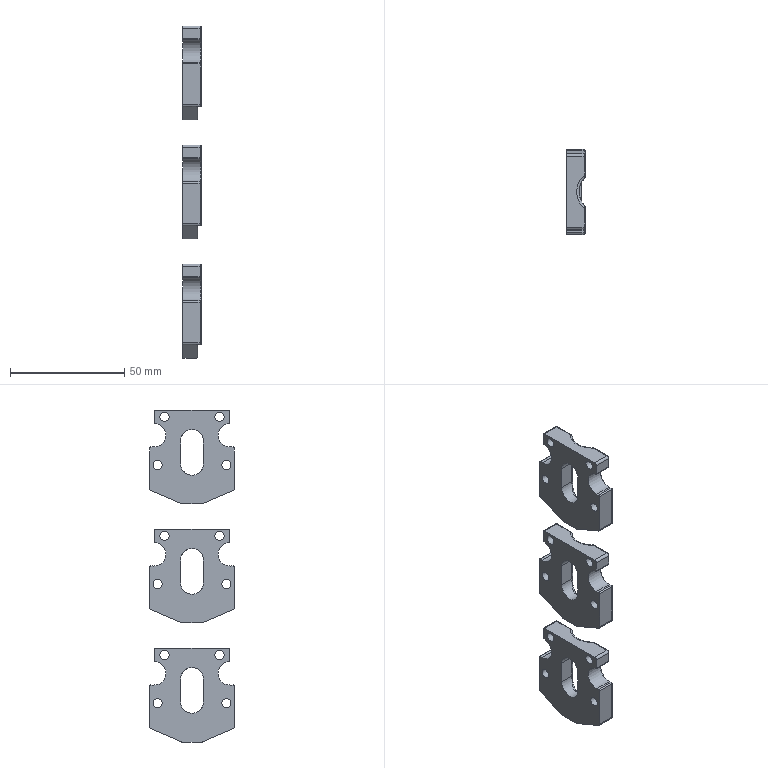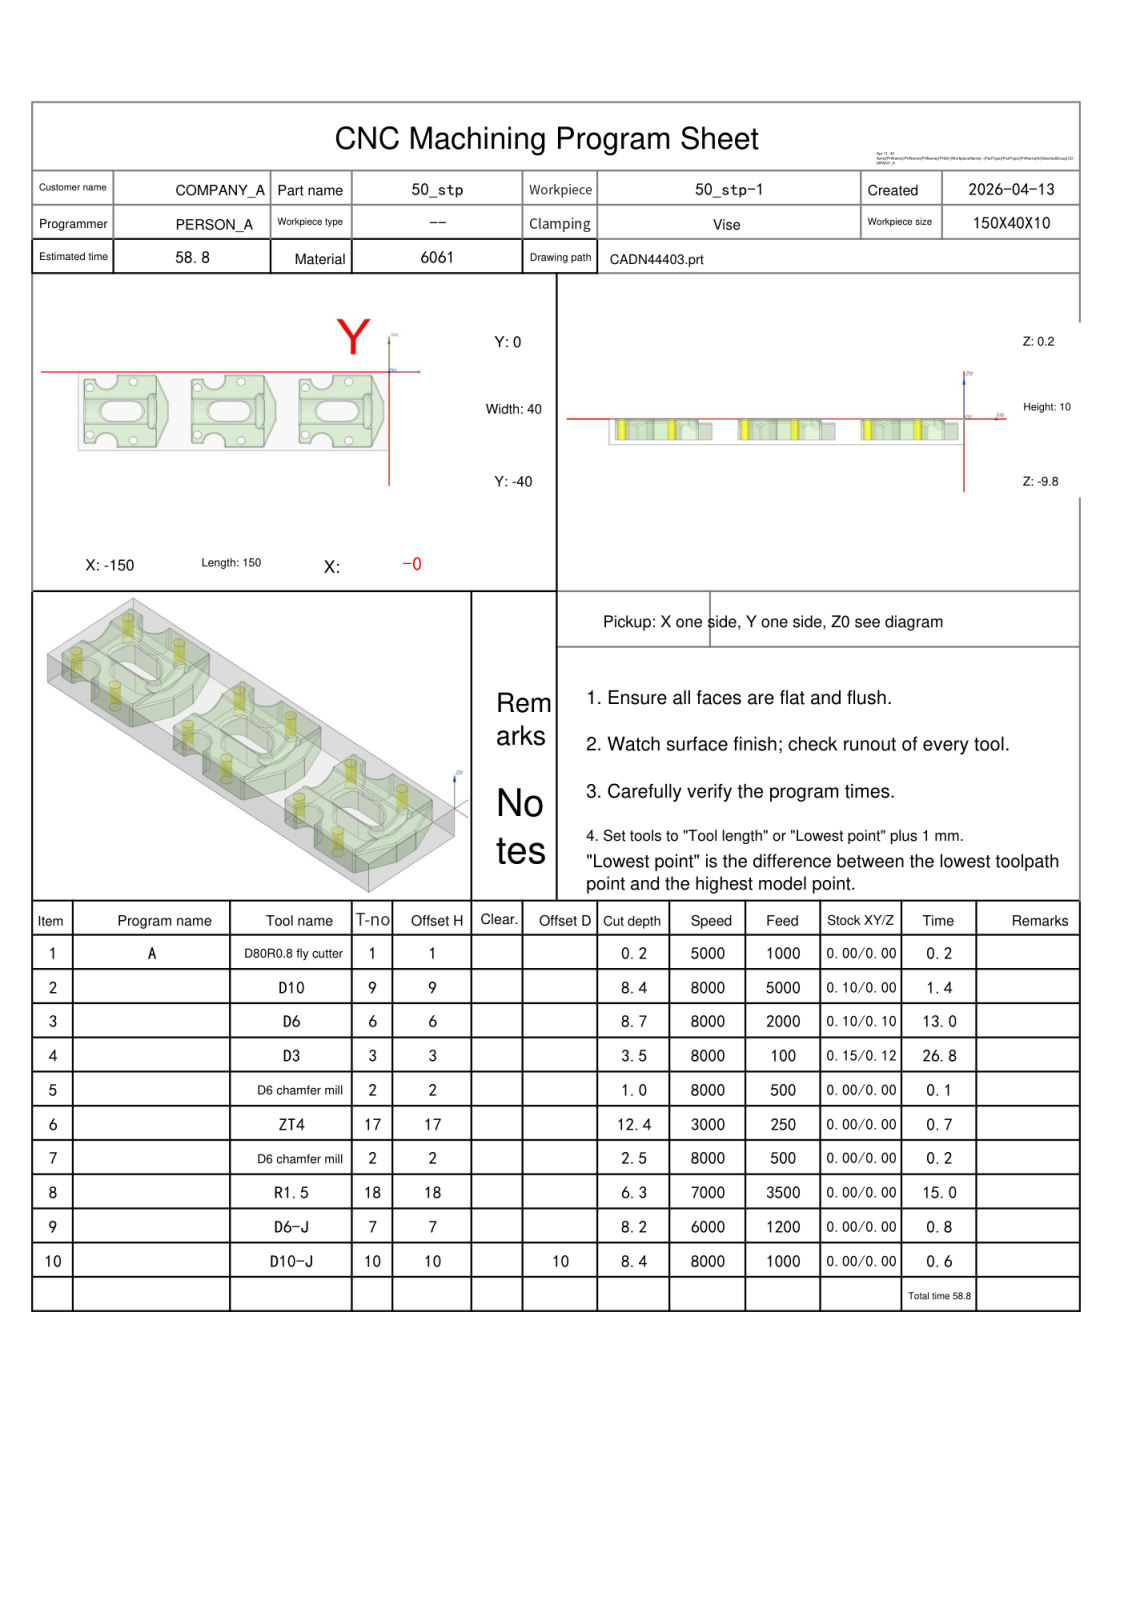NC program | NX | posted by the shop | part box 8 x 37 x 145 mm
Lines 15399 to 16378 of 223411:
N4 T03 M06
(D3  D=3. R=0. H=03 ce=0.15 di=0.12)
G00 G90 G54 X-112.073 Y-14.319 M03 S8000
G43 H03 Z10.15
M08
Z.405
G01 Z-.095 F100.
G03 X-113.572 Y-12.853 I-1.5 J-.034
G01 X-114.3
G03 X-114.703 Y-13.422 I.341 J-.668
G02 X-114.826 Y-13.87 I-3.495 J.718
G03 X-114.908 Y-14.36 I1.418 J-.49
X-114.117 Y-15.682 I1.5 J0.0
G01 Z.405
G00 Z3.
G01 X-111.94 Y-14.368 F6000.
G00 Z.31
G01 Z-.19 F100.
G03 X-113.439 Y-12.924 I-1.499 J-.057
G01 X-114.306
G03 X-114.705 Y-13.731 I.775 J-.885
G01 X-114.72 Y-13.816
G03 X-114.748 Y-14.107 I1.471 J-.291
X-113.834 Y-15.488 I1.5 J0.0
G01 Z.31
G00 Z2.905
G01 X-111.919 Y-14.435 F6000.
G00 Z.215
G01 Z-.285 F100.
G03 X-113.418 Y-12.994 I-1.499 J-.059
G01 X-114.298
G03 X-114.581 Y-13.422 I.509 J-.643
G01 X-114.698 Y-13.877
G03 X-114.745 Y-14.251 I1.453 J-.374
X-113.843 Y-15.626 I1.5 J0.0
G01 Z.215
G00 Z2.81
G01 X-112.162 Y-14.542 F6000.
G00 Z.12
G01 Z-.38 F100.
G03 X-113.662 Y-13.065 I-1.5 J-.023
G01 X-114.3
G03 X-114.663 Y-13.852 I.965 J-.922
G01 X-114.671 Y-14.004
G03 X-113.644 Y-15.428 I1.5 J0.0
G01 Z.12
G00 Z2.715
G01 X-111.678 Y-14.54 F6000.
G00 Z.025
G01 Z-.475 F100.
G03 X-113.175 Y-13.138 I-1.497 J-.098
G01 X-114.3
G03 X-114.635 Y-13.846 I.905 J-.861
G02 X-114.675 Y-14.063 I-2.625 J.378
G03 X-114.713 Y-14.399 I1.462 J-.336
X-113.808 Y-15.776 I1.5 J0.0
G01 Z.025
G00 Z2.62
G01 X-112.076 Y-14.687 F6000.
G00 Z-.07
G01 Z-.57 F100.
G03 X-113.576 Y-13.213 I-1.5 J-.026
G01 X-114.3
G03 X-114.607 Y-13.846 I.884 J-.82
G01 X-114.645 Y-14.013
G03 X-114.681 Y-14.34 I1.464 J-.327
X-113.696 Y-15.749 I1.5 J0.0
G01 Z-.07
G00 Z2.525
G01 X-112.279 Y-14.78 F6000.
G00 Z-.165
G01 Z-.665 F100.
G03 X-113.779 Y-13.29 I-1.5 J-.01
G01 X-114.254
G03 X-114.578 Y-13.846 I.496 J-.661
G01 X-114.594 Y-13.952
G03 X-114.616 Y-14.207 I1.478 J-.255
X-113.595 Y-15.629 I1.5 J0.0
G01 Z-.165
G00 Z2.43
G01 X-111.613 Y-14.745 F6000.
G00 Z-.26
G01 Z-.76 F100.
G03 X-113.107 Y-13.376 I-1.494 J-.131
G01 X-114.274
G03 X-114.593 Y-13.946 I1.157 J-1.022
G01 X-114.65 Y-14.212
X-114.656 Y-14.271
G02 X-114.763 Y-14.734 I-2.214 J.269
G03 X-114.846 Y-15.227 I1.417 J-.493
X-114.108 Y-16.519 I1.5 J0.0
G01 Z-.26
G00 Z2.335
G01 X-111.422 Y-14.809 F6000.
G00 Z-.355
G01 Z-.855 F100.
G03 X-112.913 Y-13.476 I-1.491 J-.166
G01 X-113.979
X-114.287 Y-13.472
G03 X-114.632 Y-14.271 I1.061 J-.933
G02 X-114.704 Y-14.623 I-2.621 J.349
G03 X-114.757 Y-15.02 I1.446 J-.397
X-113.91 Y-16.371 I1.5 J0.0
G01 Z-.355
G00 Z2.24
G01 X-109.207 Y-12.251 F6000.
G00 Z-.45
G01 Z-.95 F100.
G03 X-109.78 Y-12.137 I-.573 J-1.386
X-111.015 Y-12.786 I0.0 J-1.5
G02 X-112.167 Y-13.603 I-1.698 J1.171
G01 X-112.5 Y-13.591
X-113.644
X-114.289 Y-13.563
G03 X-114.609 Y-14.271 I.917 J-.841
G02 X-114.679 Y-14.618 I-3.409 J.509
G03 X-114.726 Y-14.991 I1.453 J-.373
X-113.815 Y-16.37 I1.5 J0.0
G01 Z-.45
G00 Z2.145
G01 X-111.691 Y-15.135 F6000.
G00 Z-.545
G01 Z-1.045 F100.
X-111.71 Y-15.004
G03 X-113.195 Y-13.718 I-1.485 J-.214
X-113.409 Y-13.733 I0.0 J-1.5
G01 X-113.436 Y-13.737
X-114.291 Y-13.652
G03 X-114.581 Y-14.271 I.881 J-.791
G02 X-114.639 Y-14.576 I-3.937 J.582
G03 X-114.676 Y-14.91 I1.462 J-.334
X-113.708 Y-16.313 I1.5 J0.0
G01 Z-.545
G00 Z2.05
G01 X-109.15 Y-11.698 F6000.
G00 Z-.64
G01 Z-1.14 F100.
G03 X-109.407 Y-11.676 I-.257 J-1.478
X-110.808 Y-12.64 I0.0 J-1.5
G02 X-111.321 Y-13.447 I-2.242 J.858
X-112.423 Y-13.903 I-1.102 J1.105
G01 X-112.5 Y-13.901
X-113.346
X-113.436 Y-13.921
X-114.292 Y-13.742
G03 X-114.65 Y-14.695 I1.567 J-1.133
G02 X-114.75 Y-15.15 I-2.534 J.317
G03 X-114.82 Y-15.603 I1.43 J-.453
X-114.008 Y-16.936 I1.5 J0.0
G01 Z-.64
G00 Z1.955
G01 X-109.437 Y-13.422 F6000.
G00 Z-.735
G01 Z-1.235 F100.
G03 X-110.228 Y-13.196 I-.79 J-1.275
X-111.286 Y-13.634 I0.0 J-1.5
G02 X-112.499 Y-14.135 I-1.213 J1.218
G01 X-113.353
G02 X-114.292 Y-13.832 I0.0 J1.608
G03 X-114.626 Y-14.695 I1.455 J-1.058
G02 X-114.712 Y-15.11 I-3.389 J.489
G03 X-114.765 Y-15.506 I1.447 J-.396
X-113.882 Y-16.873 I1.5 J0.0
G01 Z-.735
G00 Z1.86
G01 X-112.717 Y-16.057 F6000.
G00 Z-.83
G01 Z-1.33 F100.
G03 X-112.675 Y-15.704 I-1.458 J.353
X-113.443 Y-14.395 I-1.5 J0.0
G01 X-114.291 Y-13.921
G03 X-114.603 Y-14.695 I1.227 J-.946
G02 X-114.672 Y-15.073 I-3.674 J.471
G03 X-114.712 Y-15.417 I1.46 J-.344
X-113.762 Y-16.813 I1.5 J0.0
G01 Z-.83
G00 Z1.765
G01 X-115.362 Y-19.956 F6000.
G00 Z-.929
G01 Z-1.429 F100.
G03 X-113.862 Y-18.456 I0.0 J1.5
G01 Y-15.844
X-113.86 Y-15.711
G03 X-114.022 Y-14.531 I-4.374 J0.0
X-114.297 Y-14.039 I-1.16 J-.325
X-114.657 Y-15.12 I1.993 J-1.265
G02 X-115.551 Y-16.809 I-2.718 J.357
X-116.686 Y-17.228 I-1.135 J1.331
G01 X-116.794 Y-17.224
G03 X-118.294 Y-18.724 I0.0 J-1.5
G01 Y-18.847
Z-.929
G00 Z1.67
G01 X-115.426 Y-19.782 F6000.
G00 Z-1.028
G01 Z-1.528 F100.
G03 X-113.926 Y-18.282 I0.0 J1.5
G01 Y-15.844
Y-15.836
G03 X-114.041 Y-14.695 I-5.707 J0.0
X-114.296 Y-14.147 I-1.32 J-.28
X-114.631 Y-15.12 I2.026 J-1.24
G02 X-115.479 Y-16.914 I-2.978 J.31
X-115.953 Y-17.248 I-1.174 J1.16
G03 X-116.817 Y-18.607 I.636 J-1.358
X-116.788 Y-18.901 I1.5 J0.0
G01 Z-1.028
G00 Z1.571
G01 X-115.449 Y-20.075 F6000.
G00 Z-1.127
G01 Z-1.627 F100.
G03 X-113.949 Y-18.575 I0.0 J1.5
G01 Y-15.657
G03 X-114.282 Y-14.274 I-3.038 J0.0
G01 X-114.308 Y-14.271
X-114.507 Y-14.695
X-114.68 Y-15.544
G02 X-115.469 Y-17.081 I-2.826 J.481
X-116.693 Y-17.592 I-1.223 J1.209
G01 X-116.794 Y-17.589
G03 X-118.295 Y-19.089 I0.0 J-1.501
G01 X-118.294 Y-19.142
Z-1.127
G00 Z1.472
G01 X-115.45 Y-20.345 F6000.
G00 Z-1.226
G01 Z-1.726 F100.
G03 X-113.95 Y-18.845 I0.0 J1.5
G01 X-113.949 Y-15.994
Y-15.807
G03 X-114.282 Y-14.401 I-3.533 J-.093
X-114.573 Y-15.12 I.91 J-.787
G02 X-115.099 Y-16.817 I-4.444 J.448
X-116.777 Y-17.788 I-1.678 J.965
G01 X-116.794
G03 X-118.294 Y-19.288 I0.0 J-1.5
G01 Y-19.291
Z-1.226
G00 Z1.373
G01 X-115.45 Y-20.496 F6000.
G00 Z-1.326
G01 Z-1.826 F100.
G03 X-113.95 Y-18.996 I0.0 J1.5
G01 Y-16.074
X-114.059 Y-15.12
X-114.282 Y-14.527
X-114.311 Y-14.522
G03 X-114.624 Y-15.544 I2.7 J-1.384
G02 X-115.449 Y-17.465 I-3.252 J.258
X-116.302 Y-17.965 I-1.207 J1.084
G03 X-117.474 Y-19.429 I.327 J-1.464
G01 X-117.472 Y-19.501
Z-1.326
G00 Z2.525
G01 X-111.599 Y-14.741 F6000.
G00 Z-.26
G01 Z-.76 F100.
X-112.853 Y-14.174
G03 X-113.471 Y-14.04 I-.619 J-1.366
X-114.838 Y-14.922 I0.0 J-1.5
G02 X-116.796 Y-16.229 I-2.031 J.922
G03 X-118.296 Y-17.729 I0.0 J-1.5
G01 Y-17.74
Z-.26
G00 Z3.
G01 X-114.081 Y-24.359 F6000.
G00 Z.405
G01 Z-.095 F100.
G03 X-114.902 Y-25.697 I.678 J-1.338
X-114.826 Y-26.171 I1.5 J0.0
G01 X-114.584 Y-26.896
X-114.349 Y-27.131
X-114.3 Y-27.147
X-113.57
G03 X-112.071 Y-25.681 I0.0 J1.5
G01 Z.405
G00 Z3.
G01 X-113.871 Y-24.459 F6000.
G00 Z.31
G01 Z-.19 F100.
G03 X-114.762 Y-25.83 I.609 J-1.371
X-114.728 Y-26.147 I1.5 J0.0
G01 X-114.695 Y-26.341
G03 X-114.3 Y-27.076 I1.143 J.141
G01 X-113.461
G03 X-111.962 Y-25.628 I0.0 J1.5
G01 Z.31
G00 Z2.905
G01 X-118.286 Y-22.261 F6000.
G00 Z-.26
G01 Z-.76 F100.
Y-22.271
G03 X-116.786 Y-23.771 I1.5 J0.0
G01 X-116.749
G02 X-114.842 Y-25.07 I-.121 J-2.228
G03 X-113.478 Y-25.946 I1.364 J.624
X-112.854 Y-25.81 I0.0 J1.5
G01 X-111.629 Y-25.25
Z-.26
G00 Z2.81
G01 X-113.777 Y-24.47 F6000.
G00 Z.215
G01 Z-.285 F100.
G03 X-114.718 Y-25.862 I.559 J-1.392
X-114.695 Y-26.126 I1.5 J0.0
G01 X-114.678 Y-26.236
G03 X-114.299 Y-27.006 I1.304 J.164
G01 X-113.439
G03 X-111.94 Y-25.561 I0.0 J1.5
G01 Z.215
G00 Z2.81
G01 X-113.713 Y-24.458 F6000.
G00 Z.12
G01 Z-.38 F100.
G03 X-114.689 Y-25.864 I.525 J-1.405
X-114.671 Y-26.093 I1.5 J0.0
G01 X-114.662 Y-26.154
G03 X-114.3 Y-26.935 I1.301 J.129
G01 X-113.602
G03 X-112.102 Y-25.463 I0.0 J1.5
G01 Z.12
G00 Z2.715
G01 X-113.812 Y-24.206 F6000.
G00 Z.025
G01 Z-.475 F100.
G03 X-114.72 Y-25.584 I.592 J-1.378
X-114.679 Y-25.933 I1.5 J0.0
G02 X-114.635 Y-26.154 I-2.825 J-.675
G03 X-114.3 Y-26.862 I1.22 J.144
G01 X-113.113
G03 X-111.618 Y-25.489 I0.0 J1.5
G01 Z.025
G00 Z2.62
G01 X-113.685 Y-24.306 F6000.
G00 Z-.07
G01 Z-.57 F100.
G03 X-114.66 Y-25.711 I.525 J-1.405
X-114.634 Y-25.993 I1.5 J0.0
G01 X-114.607 Y-26.154
G03 X-114.3 Y-26.787 I1.185 J.183
G01 X-113.577
G03 X-112.077 Y-25.318 I0.0 J1.5
G01 Z-.07
G00 Z2.525
G01 X-113.6 Y-24.361 F6000.
G00 Z-.165
G01 Z-.665 F100.
G03 X-114.618 Y-25.781 I.482 J-1.42
X-114.596 Y-26.041 I1.5 J0.0
G01 X-114.578 Y-26.154
G03 X-114.254 Y-26.71 I.817 J.103
G01 X-113.771
G03 X-112.271 Y-25.22 I0.0 J1.5
G01 Z-.165
G00 Z2.43
G01 X-114.106 Y-23.483 F6000.
G00 Z-.26
G01 Z-.76 F100.
G03 X-114.846 Y-24.776 I.76 J-1.293
X-114.763 Y-25.268 I1.5 J0.0
G02 X-114.656 Y-25.729 I-2.108 J-.731
G01 X-114.649 Y-25.791
X-114.595 Y-26.047
G03 X-114.285 Y-26.615 I1.52 J.459
G01 X-113.859 Y-26.624
X-113.199
G03 X-111.703 Y-25.23 I0.0 J1.5
G01 Z-.26
G00 Z2.335
G01 X-113.909 Y-23.613 F6000.
G00 Z-.355
G01 Z-.855 F100.
G03 X-114.767 Y-24.968 I.642 J-1.356
X-114.71 Y-25.378 I1.5 J0.0
G02 X-114.633 Y-25.729 I-2.929 J-.831
G03 X-114.287 Y-26.528 I1.409 J.136
G01 X-113.859 Y-26.516
X-113.794 Y-26.524
X-113.209
G03 X-111.712 Y-25.133 I0.0 J1.5
G01 Z-.355
G00 Z2.24
G01 X-113.813 Y-23.634 F6000.
G00 Z-.45
G01 Z-.95 F100.
G03 X-114.726 Y-25.014 I.587 J-1.38
X-114.679 Y-25.386 I1.5 J0.0
G02 X-114.609 Y-25.729 I-3.365 J-.862
G03 X-114.289 Y-26.437 I1.238 J.133
G01 X-113.614 Y-26.387
X-113.588 Y-26.409
X-112.5
G02 X-110.883 Y-27.437 I-.006 J-1.795
G03 X-109.521 Y-28.309 I1.362 J.628
X-109.154 Y-28.264 I0.0 J1.5
G01 Z-.45
G00 Z2.145
G01 X-113.701 Y-23.701 F6000.
G00 Z-.545
G01 Z-1.045 F100.
G03 X-114.673 Y-25.105 I.527 J-1.404
X-114.636 Y-25.436 I1.5 J0.0
G02 X-114.581 Y-25.729 I-3.903 J-.883
G03 X-114.291 Y-26.348 I1.171 J.173
G01 X-113.436 Y-26.263
X-113.392 Y-26.269
G03 X-113.18 Y-26.284 I.212 J1.485
X-111.695 Y-24.996 I0.0 J1.5
G01 X-111.677 Y-24.872
Z-.545
G00 Z2.05
G01 X-114.073 Y-22.957 F6000.
G00 Z-.64
G01 Z-1.14 F100.
G03 X-114.877 Y-24.286 I.695 J-1.329
X-114.793 Y-24.781 I1.5 J0.0
G02 X-114.551 Y-25.729 I-5.379 J-1.882
G03 X-114.292 Y-26.258 I1.065 J.193
G01 X-113.436 Y-26.073
X-113.301 Y-26.099
X-112.499
G02 X-110.901 Y-27.143 I0.0 J-1.744
G01 X-110.834 Y-27.312
G03 X-109.426 Y-28.294 I1.408 J.518
X-109.15 Y-28.268 I0.0 J1.5
G01 Z-.64
G00 Z1.955
G01 X-113.912 Y-23.087 F6000.
G00 Z-.735
G01 Z-1.235 F100.
G03 X-114.778 Y-24.446 I.635 J-1.359
X-114.72 Y-24.856 I1.5 J0.0
G02 X-114.626 Y-25.305 I-3.135 J-.892
G01 X-114.605 Y-25.448
X-114.59 Y-25.515
G03 X-114.292 Y-26.168 I1.756 J.407
G02 X-113.375 Y-25.865 I.918 J-1.239
G01 X-112.355
G02 X-111.477 Y-26.172 I0.0 J-1.413
G03 X-110.544 Y-26.497 I.933 J1.175
X-109.619 Y-26.179 I0.0 J1.5
G01 Z-.735
G00 Z1.86
G01 X-113.784 Y-23.15 F6000.
G00 Z-.83
G01 Z-1.33 F100.
G03 X-114.722 Y-24.541 I.562 J-1.391
X-114.679 Y-24.897 I1.5 J0.0
G02 X-114.603 Y-25.305 I-3.598 J-.879
G03 X-114.291 Y-26.079 I1.54 J.172
G01 X-113.425 Y-25.6
G03 X-112.651 Y-24.288 I-.726 J1.313
X-112.691 Y-23.943 I-1.5 J0.0
G01 Z-.83
G00 Z1.765
G01 X-118.287 Y-21.146 F6000.
G00 Z-.929
G01 Z-1.429 F100.
Y-21.276
G03 X-116.787 Y-22.776 I1.5 J0.0
G01 X-116.749
X-116.735
G02 X-115.259 Y-23.487 I0.0 J-1.888
X-114.657 Y-24.88 I-2.266 J-1.806
G03 X-114.296 Y-25.962 I2.35 J.183
X-114.011 Y-25.443 I-.856 J.809
X-113.861 Y-24.243 I-4.718 J1.2
G01 X-113.862 Y-24.156
Y-21.55
G03 X-115.362 Y-20.05 I-1.5 J0.0
G01 Z-.929
G00 Z1.67
G01 X-116.962 Y-21.099 F6000.
G00 Z-1.028
G01 Z-1.528 F100.
G03 X-116.982 Y-21.343 I1.48 J-.244
X-116.038 Y-22.736 I1.5 J0.0
G02 X-115.059 Y-23.607 I-.713 J-1.788
X-114.631 Y-24.88 I-3.046 J-1.733
G03 X-114.31 Y-25.835 I2.457 J.293
X-114.065 Y-25.437 I-.463 J.559
X-113.926 Y-24.192 I-5.484 J1.245
G01 Y-24.156
Y-21.72
G03 X-115.426 Y-20.22 I-1.5 J0.0
G01 Z-1.028
G00 Z1.571
G01 X-118.288 Y-20.767 F6000.
G00 Z-1.127
G01 Z-1.627 F100.
Y-20.911
G03 X-116.788 Y-22.411 I1.5 J0.0
G01 X-116.749
X-116.725
G02 X-115.245 Y-23.183 I0.0 J-1.806
X-114.604 Y-24.88 I-2.663 J-1.974
G03 X-114.311 Y-25.725 I2.106 J.259
G01 X-114.285 Y-25.729
G03 X-113.949 Y-24.355 I-2.647 J1.375
G01 Y-21.417
G03 X-115.449 Y-19.917 I-1.5 J0.0
G01 Z-1.127
G00 Z1.472
G01 X-118.288 Y-20.709 F6000.
G00 Z-1.226
G01 Z-1.726 F100.
Y-20.712
G03 X-116.788 Y-22.212 I1.5 J0.0
G01 X-116.749
G02 X-115.099 Y-23.183 I-.028 J-1.936
X-114.573 Y-24.88 I-3.918 J-2.145
G03 X-114.282 Y-25.599 I1.201 J.068
X-113.949 Y-24.182 I-3.223 J1.504
G01 X-113.95 Y-23.979
Y-21.083
G03 X-115.45 Y-19.583 I-1.5 J0.0
G01 Z-1.226
G00 Z1.373
G01 X-117.532 Y-20.499 F6000.
G00 Z-1.326
G01 Z-1.826 F100.
X-117.534 Y-20.578
G03 X-116.359 Y-22.042 I1.5 J0.0
G02 X-115.328 Y-22.684 I-.396 J-1.784
X-114.624 Y-24.456 I-2.54 J-2.035
G03 X-114.311 Y-25.478 I3.012 J.362
G01 X-114.282 Y-25.473
X-114.059 Y-24.88
X-113.958 Y-24.032
X-113.95 Y-23.926
Y-20.741
G03 X-115.45 Y-19.241 I-1.5 J0.0
G01 Y-19.393
Z-1.326
G00 Z1.274
G01 X-119.548 Y-20. F6000.
G00 Z-1.425
G01 Z-1.925 F100.
X-118.783 Y-19.823
G02 X-117.421 Y-18.952 I1.361 J-.63
X-116.792 Y-19.091 I0.0 J-1.5
G01 X-114.482 Y-20.159
G02 X-114.046 Y-20.84 I-.315 J-.681
X-114.796 Y-21.59 I-.75 J0.0
X-115.111 Y-21.521 I0.0 J.75
G01 X-116.543 Y-20.859
X-116.656 Y-20.834
G03 X-116.902 Y-20.992 I0.0 J-.27
G01 X-117.062 Y-21.345
X-117.088 Y-21.469
G03 X-116.788 Y-21.769 I.3 J0.0
G01 X-116.749
G02 X-115.128 Y-22.707 I-.032 J-1.926
X-114.595 Y-24.456 I-3.782 J-2.109
G03 X-114.312 Y-25.355 I2.386 J.257
G01 X-114.282 Y-25.346
X-114.103 Y-24.88
G03 X-113.95 Y-23.767 I-7.84 J1.642
G01 Y-16.233
G03 X-114.103 Y-15.12 I-8.037 J-.535
G01 X-114.282 Y-14.654
X-114.312 Y-14.645
G03 X-114.595 Y-15.544 I2.103 J-1.156
G02 X-115.128 Y-17.293 I-4.315 J.36
X-116.782 Y-18.231 I-1.654 J.988
G01 X-116.793
G03 X-118.293 Y-19.731 I0.0 J-1.5
G01 X-119.548 Y-20.
Z-1.425
G00 Z1.174
Z-1.524
G01 X-119.549 Z-2.024
X-117.957 Y-20.995
G02 X-117.988 Y-20.691 I1.469 J.303
X-116.792 Y-19.222 I1.5 J0.0
G01 X-114.897 Y-18.831
X-114.745 Y-18.815
G02 X-113.995 Y-19.565 I0.0 J-.75
X-114.593 Y-20.3 I-.75 J0.0
G01 X-116.688 Y-20.733
X-116.796 Y-20.743
X-116.857 Y-20.833
X-117.018 Y-21.025
G03 X-117.089 Y-21.218 I.229 J-.193
X-116.789 Y-21.518 I.3 J0.0
G01 X-116.749
G02 X-115.35 Y-22.201 I-.009 J-1.793
X-114.635 Y-24.032 I-2.656 J-2.092
G03 X-114.312 Y-25.223 I3.647 J.35
G01 X-114.282 Y-25.212
X-114.155 Y-24.88
G03 X-113.95 Y-23.555 I-5.26 J1.492
G01 Y-16.445
G03 X-114.155 Y-15.12 I-5.449 J-.164
G01 X-114.282 Y-14.788
X-114.312 Y-14.777
G03 X-114.635 Y-15.968 I3.324 J-1.541
G02 X-115.35 Y-17.799 I-3.371 J.262
X-116.758 Y-18.482 I-1.409 J1.109
G01 X-116.793
G03 X-118.293 Y-19.982 I0.0 J-1.5
G01 X-119.549 Y-20.
Z-1.524
G00 Z1.075
G01 X-120.764 Y-20.002 F6000.
G00 Z-1.623
G01 Z-2.123 F100.
X-118.289 Y-19.741
G03 X-116.789 Y-21.241 I1.5 J0.0
G01 X-116.749
X-116.744
G02 X-115.128 Y-22.232 I0.0 J-1.813
X-114.606 Y-24.032 I-4.049 J-2.149
G03 X-114.312 Y-25.086 I3.42 J.388
G01 X-114.282 Y-25.075
X-114.069 Y-24.456
G03 X-113.95 Y-23.289 I-10.74 J1.687
G01 Y-16.711
G03 X-114.069 Y-15.544 I-10.768 J-.511
G01 X-114.282 Y-14.925
X-114.312 Y-14.914
G03 X-114.606 Y-15.968 I3.126 J-1.442
G02 X-115.128 Y-17.768 I-4.57 J.349
X-116.036 Y-18.615 I-1.616 J.822
G03 X-116.219 Y-18.891 I.117 J-.276
X-116.135 Y-19.098 I.3 J0.0
G02 X-115.829 Y-19.862 I-.799 J-.764
G01 X-115.834 Y-19.965
X-115.835 Y-20.
G03 X-115.606 Y-20.346 I.375 J0.0
G01 X-115.45 Y-20.379
G03 X-115.075 Y-20.004 I0.0 J.375
G01 Y-19.996
G03 X-115.383 Y-19.627 I-.375 J0.0
G02 X-115.605 Y-19.369 I.048 J.266
G01 X-115.619 Y-18.882
G03 X-115.918 Y-18.591 I-.3 J-.009
G01 X-116.036 Y-18.615
G02 X-116.745 Y-18.759 I-.709 J1.669
G01 X-116.792
G03 X-118.292 Y-20.259 I0.0 J-1.5
G01 X-120.764 Y-20.021
Z-1.623
G00 Z.976
G01 X-120.763 Y-19.986 F6000.
G00 Z-1.722
G01 Z-2.222 F100.
X-118.29 Y-19.43
G03 X-116.79 Y-20.93 I1.5 J0.0
G01 X-116.749
G02 X-115.229 Y-21.776 I-.007 J-1.803
X-114.638 Y-23.607 I-3.329 J-2.084
G03 X-114.312 Y-24.948 I4.215 J.315
G01 X-114.282 Y-24.938
X-114.12 Y-24.456
G03 X-113.95 Y-23.078 I-6.332 J1.479
G01 Y-16.909
G03 X-114.225 Y-15.231 I-5.257 J0.0
G01 X-114.282 Y-15.062
X-114.312 Y-15.052
G03 X-114.638 Y-16.393 I3.888 J-1.657
G02 X-115.427 Y-18.473 I-3.59 J.172
X-116.681 Y-19.074 I-1.254 J1.006
G01 X-116.792 Y-19.07
G03 X-118.292 Y-20.57 I0.0 J-1.5
G01 X-120.762 Y-20.027
Z-1.722
G00 Z.877
G01 X-120.983 Y-20. F6000.
G00 Z-1.821
G01 Z-2.321 F100.
X-117.54 Y-19.818
G03 X-116.79 Y-20.568 I.75 J0.0
G01 X-116.749
X-116.668 Y-20.566
G02 X-115.317 Y-21.309 I0.0 J-1.599
X-114.665 Y-23.183 I-3.681 J-2.332
G03 X-114.312 Y-24.801 I5.815 J.421
X-114.028 Y-23.815 I-2.299 J1.196
G01 X-113.95 Y-22.758
Y-17.242
X-114.028 Y-16.185
X-114.054 Y-15.998
X-114.282 Y-15.211
X-114.312 Y-15.199
G03 X-114.665 Y-16.817 I5.473 J-2.042
G02 X-115.551 Y-18.962 I-3.771 J.302
X-116.58 Y-19.443 I-1.029 J.861
G01 X-116.749 Y-19.432
X-116.791
G03 X-117.541 Y-20.182 I0.0 J-.75
G01 X-120.983 Y-20.
Z-1.821
G00 Z.778
G01 X-121.267 Y-20.005 F6000.
G00 Z-1.92
G01 Z-2.42 F100.
X-117.321 Y-19.903
G03 X-116.791 Y-20.123 I.53 J.53
G01 X-116.749
G02 X-115.128 Y-21.208 I-.039 J-1.813
X-114.633 Y-23.183 I-5.899 J-2.527
G03 X-114.312 Y-24.643 I5.107 J.358
G01 X-114.282 Y-24.631
X-114.073 Y-23.918
X-114.048 Y-23.761
X-114.029 Y-23.607
X-113.95 Y-22.493
Y-17.507
X-114.029 Y-16.393
X-114.047 Y-16.24
X-114.073 Y-16.082
X-114.282 Y-15.369
X-114.312 Y-15.357
G03 X-114.633 Y-16.817 I4.805 J-1.823
G02 X-115.128 Y-18.792 I-6.379 J.548
X-116.789 Y-19.877 I-1.661 J.728
G01 X-116.791
G03 X-117.321 Y-20.097 I0.0 J-.75
G01 X-121.267 Y-20.01
Z-1.92
G00 Z.679
G01 X-114.499 Y-19.031 F6000.
G00 Z-1.82
G01 X-114.629 Y-19.432 Z-1.842 F100.
X-114.663 Y-19.506 Z-1.847
X-114.958 Y-20.004 Z-1.877
X-114.663 Y-20.498 Z-1.907
X-114.629 Y-20.573 Z-1.911
X-114.45 Y-21.121 Z-1.942
Y-18.881 Z-2.059
X-114.629 Y-19.432 Z-2.089
X-114.663 Y-19.506 Z-2.094
X-114.958 Y-20.004 Z-2.124
X-114.663 Y-20.498 Z-2.154
X-114.629 Y-20.573 Z-2.158
X-114.45 Y-21.121 Z-2.189
Y-18.881 Z-2.306
X-114.629 Y-19.432 Z-2.336
X-114.663 Y-19.506 Z-2.341
X-114.958 Y-20.004 Z-2.371
X-114.663 Y-20.498 Z-2.401
X-114.629 Y-20.573 Z-2.405
X-114.45 Y-21.121 Z-2.436
Y-19.522 Z-2.519
X-113.95
Y-17.878
G03 X-114.107 Y-16.084 I-13.747 J-.299
G01 X-114.282 Y-15.526
X-114.312 Y-15.515
G03 X-114.69 Y-17.518 I8.428 J-2.627
G02 X-115.551 Y-20.004 I-5.058 J.358
X-114.69 Y-22.479 I-4.142 J-2.828
G03 X-114.312 Y-24.485 I8.809 J.622
X-114.048 Y-23.549 I-2.264 J1.143
G01 X-114.025 Y-23.338
X-113.95 Y-22.122
Y-19.522
Y-19.222
G03 X-114.7 Y-18.472 I-.75 J0.0
G01 Z-2.019
G00 Z1.373
G01 X-114.032 Y-23.174 F6000.
G00 Z-1.919
G01 X-114.068 Y-23.666 Z-1.945 F100.
X-114.12 Y-23.89 Z-1.957
X-114.3 Y-24.34 Z-1.983
X-114.483 Y-23.856 Z-2.01
X-114.519 Y-23.698 Z-2.018
X-114.568 Y-23.183 Z-2.045
X-114.672 Y-22.006 Z-2.107
X-114.682 Y-21.932 Z-2.111
X-114.908 Y-20.772 Z-2.173
X-114.682 Y-21.932 Z-2.235
X-114.672 Y-22.006 Z-2.239
X-114.568 Y-23.183 Z-2.301
X-114.519 Y-23.698 Z-2.328
X-114.483 Y-23.856 Z-2.337
X-114.3 Y-24.34 Z-2.364
X-114.12 Y-23.89 Z-2.389
X-114.068 Y-23.666 Z-2.401
X-114.032 Y-23.183 Z-2.427
X-113.95 Y-21.645 Z-2.507
Y-19.522 Z-2.619
Y-18.355
X-114.032 Y-16.817
X-114.074 Y-16.505
G03 X-114.3 Y-15.66 I-3.351 J-.442
X-114.568 Y-16.817 I4.172 J-1.578
G02 X-114.935 Y-19.363 I-23.06 J2.026
G01 Y-20.637
G02 X-114.568 Y-23.183 I-22.8 J-4.59
G03 X-114.3 Y-24.34 I4.42 J.415
X-114.032 Y-23.183 I-3.613 J1.444
G01 X-113.95 Y-21.645
Y-19.522
Y-19.222
G03 X-114.7 Y-18.472 I-.75 J0.0
G01 Z-2.119
G00 Z1.373
G01 X-114.043 Y-23.169 F6000.
G00 Z-2.019
G01 X-114.051 Y-23.334 Z-2.027 F100.
X-114.118 Y-23.668 Z-2.045
X-114.299 Y-24.164 Z-2.073
X-114.488 Y-23.603 Z-2.104
X-114.54 Y-23.348 Z-2.117
X-114.586 Y-22.758 Z-2.148
X-114.702 Y-21.58 Z-2.21
X-114.826 Y-20.403 Z-2.272
X-114.702 Y-21.58 Z-2.335
X-114.586 Y-22.758 Z-2.397
X-114.54 Y-23.348 Z-2.428
X-114.488 Y-23.603 Z-2.441
X-114.299 Y-24.164 Z-2.472
X-114.118 Y-23.668 Z-2.5
X-114.051 Y-23.334 Z-2.518
X-114.025 Y-22.807 Z-2.545
X-113.95 Y-21.167 Z-2.631
Y-19.522 Z-2.718
Y-18.833
X-114.025 Y-17.193
X-114.05 Y-16.929
G03 X-114.299 Y-15.836 I-4.154 J-.373
X-114.667 Y-18.09 I8.855 J-2.602
X-114.847 Y-20.212 I27.232 J-3.37
G02 X-114.586 Y-22.758 I-323.808 J-34.42
G03 X-114.299 Y-24.164 I5.801 J.451
X-114.025 Y-22.807 I-4.355 J1.588
G01 X-113.95 Y-21.167
Y-19.522
Y-19.222
G03 X-114.7 Y-18.472 I-.75 J0.0
G01 Z-2.218
G00 Z.381
G01 X-114.066 Y-23.171 F6000.
G00 Z-2.118
G01 X-114.118 Y-23.449 Z-2.132 F100.
X-114.298 Y-23.982 Z-2.162
X-114.478 Y-23.438 Z-2.192
X-114.501 Y-23.33 Z-2.198
X-114.552 Y-22.758 Z-2.228
X-114.597 Y-22.334 Z-2.25
X-114.722 Y-21.162 Z-2.312
X-114.724 Y-20.027 Z-2.371
X-114.72 Y-21.206 Z-2.433
X-114.597 Y-22.334 Z-2.493
X-114.552 Y-22.758 Z-2.515
X-114.501 Y-23.33 Z-2.545
X-114.478 Y-23.438 Z-2.551
X-114.298 Y-23.982 Z-2.581
X-114.118 Y-23.449 Z-2.61
X-114.054 Y-23.106 Z-2.629
X-114.028 Y-22.544 Z-2.658
X-113.943 Y-21.034 Z-2.738
X-113.959 Y-19.522 Z-2.817
G03 X-114.028 Y-17.456 I-44.968 J-.478
X-114.298 Y-16.017 I-5.39 J-.265
X-114.553 Y-17.242 I5.224 J-1.726
G01 X-114.596 Y-17.666
G03 X-114.724 Y-20.006 I21.314 J-2.34
X-114.597 Y-22.334 I21.442 J0.0
G01 X-114.552 Y-22.758
G03 X-114.298 Y-23.982 I5.444 J.493
X-114.028 Y-22.544 I-4.987 J1.679
X-113.956 Y-20. I-44.898 J2.544
X-113.959 Y-19.522 I-44.97 J0.0
X-113.963 Y-19.222 I-44.968 J-.478
X-114.192 Y-18.696 I-.75 J-.013
G01 Z-2.317
G00 Z.282
G01 X-114.113 Y-23.166 F6000.
G00 Z-2.217
G01 X-114.298 Y-23.785 Z-2.251 F100.
X-114.48 Y-23.169 Z-2.284
X-114.516 Y-22.976 Z-2.295
X-114.563 Y-22.334 Z-2.328
X-114.68 Y-21.143 Z-2.391
X-114.693 Y-20.822 Z-2.408
X-114.674 Y-19.625 Z-2.471
X-114.693 Y-20.822 Z-2.533
X-114.68 Y-21.143 Z-2.55
X-114.563 Y-22.334 Z-2.613
X-114.516 Y-22.976 Z-2.647
X-114.48 Y-23.169 Z-2.657
X-114.298 Y-23.785 Z-2.691
X-114.117 Y-23.192 Z-2.723
X-114.074 Y-22.953 Z-2.736
X-114.035 Y-22.334 Z-2.768
X-113.963 Y-20.929 Z-2.842
X-113.977 Y-19.522 Z-2.916
G03 X-114.035 Y-17.666 I-45.569 J-.478
X-114.298 Y-16.215 I-6.351 J-.401
X-114.552 Y-17.567 I7.917 J-2.191
X-114.677 Y-20.004 I23.75 J-2.437
X-114.563 Y-22.334 I23.875 J0.0
X-114.298 Y-23.785 I6.867 J.506
X-114.035 Y-22.334 I-6.128 J1.86
X-113.975 Y-20. I-45.512 J2.334
X-113.977 Y-19.522 I-45.572 J0.0
X-113.981 Y-19.222 I-45.569 J-.478
X-114.21 Y-18.696 I-.75 J-.013
G01 Z-2.416
G00 Z.183
G01 X-114.179 Y-23.156 F6000.
G00 Z-2.316
G01 X-114.298 Y-23.576 Z-2.339 F100.
X-114.485 Y-22.822 Z-2.379
X-114.654 Y-20.864 Z-2.482
X-114.666 Y-20.398 Z-2.507
X-114.626 Y-19.197 Z-2.57
X-114.666 Y-20.398 Z-2.633
X-114.654 Y-20.864 Z-2.657
X-114.551 Y-22.061 Z-2.72
X-114.483 Y-22.835 Z-2.761
X-114.298 Y-23.576 Z-2.801
X-114.123 Y-22.963 Z-2.834
X-114.088 Y-22.755 Z-2.845
X-114.05 Y-22.119 Z-2.879
X-113.979 Y-20.822 Z-2.947
X-113.995 Y-19.523 Z-3.015
G03 X-114.05 Y-17.881 I-38.295 J-.477
X-114.298 Y-16.424 I-6.73 J-.397
X-114.551 Y-17.935 I9.335 J-2.335
X-114.639 Y-19.998 I23.977 J-2.063
X-114.551 Y-22.061 I24.065 J0.0
X-114.298 Y-23.576 I9.671 J.832
X-114.05 Y-22.119 I-6.488 J1.854
X-113.992 Y-20. I-38.239 J2.119
X-113.995 Y-19.523 I-38.298 J0.0
X-114. Y-19.223 I-38.295 J-.477
X-114.23 Y-18.697 I-.75 J-.015
G01 Z-2.515
G00 Z.084
G01 X-114.248 Y-23.148 F6000.
G00 Z-2.415
G01 X-114.299 Y-23.349 Z-2.426 F100.
X-114.491 Y-22.434 Z-2.475
X-114.637 Y-20.722 Z-2.565
X-114.601 Y-19.788 Z-2.614
X-114.611 Y-19.262 Z-2.641
X-114.581 Y-18.737 Z-2.669
X-114.611 Y-19.262 Z-2.697
X-114.601 Y-19.788 Z-2.724
X-114.637 Y-20.722 Z-2.773
X-114.491 Y-22.434 Z-2.863
X-114.299 Y-23.349 Z-2.912
X-114.122 Y-22.647 Z-2.95
X-114.06 Y-22.209 Z-2.973
X-114.038 Y-21.485 Z-3.011
X-113.993 Y-20.505 Z-3.063
X-114.012 Y-19.523 Z-3.114
G03 X-114.105 Y-17.666 I-30.303 J-.585
G01 X-114.124 Y-17.513
X-114.282 Y-16.709
X-114.299 Y-16.651
G03 X-114.603 Y-19.517 I13.323 J-2.866
X-114.601 Y-19.788 I13.628 J0.0
X-114.611 Y-20.348 I14.535 J-.56
X-114.299 Y-23.349 I14.546 J0.0
X-114.038 Y-21.485 I-8.457 J2.132
X-114.007 Y-20.108 I-30.278 J1.378
X-114.012 Y-19.523 I-30.309 J0.0
X-114.02 Y-19.223 I-30.303 J-.585
X-114.255 Y-18.699 I-.75 J-.022
G01 Z-2.614
G00 Z-.015
G01 X-114.31 Y-23.046 F6000.
G00 Z-2.514
G01 X-114.478 Y-22.219 Z-2.558 F100.
X-114.581 Y-21.108 Z-2.617
X-114.566 Y-20.212 Z-2.664
X-114.597 Y-19.274 Z-2.713
X-114.593 Y-19.162 Z-2.719
X-114.497 Y-18.228 Z-2.768
X-114.593 Y-19.162 Z-2.817
X-114.597 Y-19.274 Z-2.823
X-114.566 Y-20.212 Z-2.872
X-114.581 Y-21.108 Z-2.919
X-114.478 Y-22.219 Z-2.978